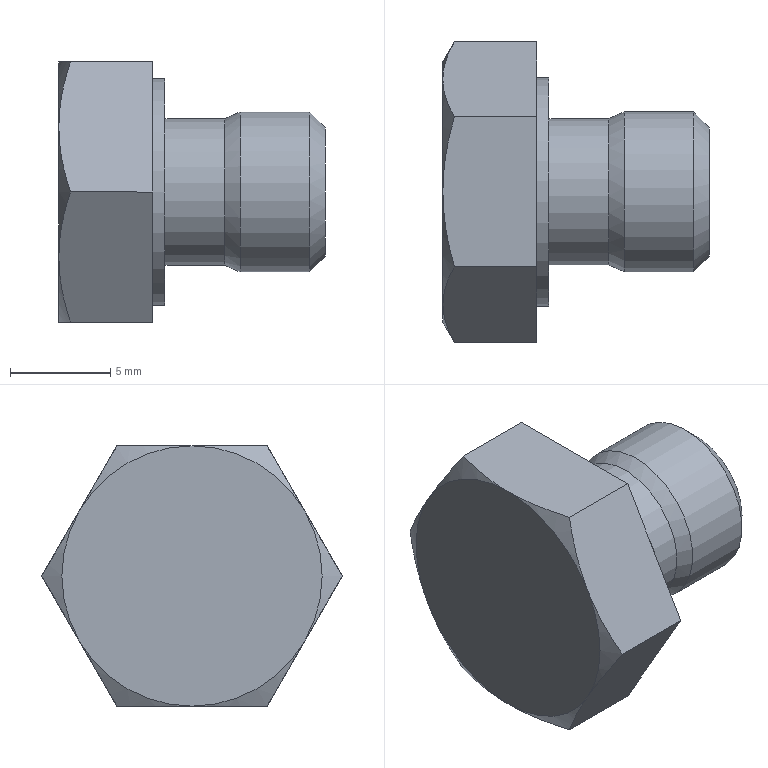Part | STEP file | DIN 933 - M8  x 8 | 1 solid | 21 faces | box 13.3 x 15.011 x 13 mm | volume 1114 mm3 | plane 10 | cone 8 | cylinder 3 | commonest cylinder face diameters 7.323 x1 8 x1 11.4 x1